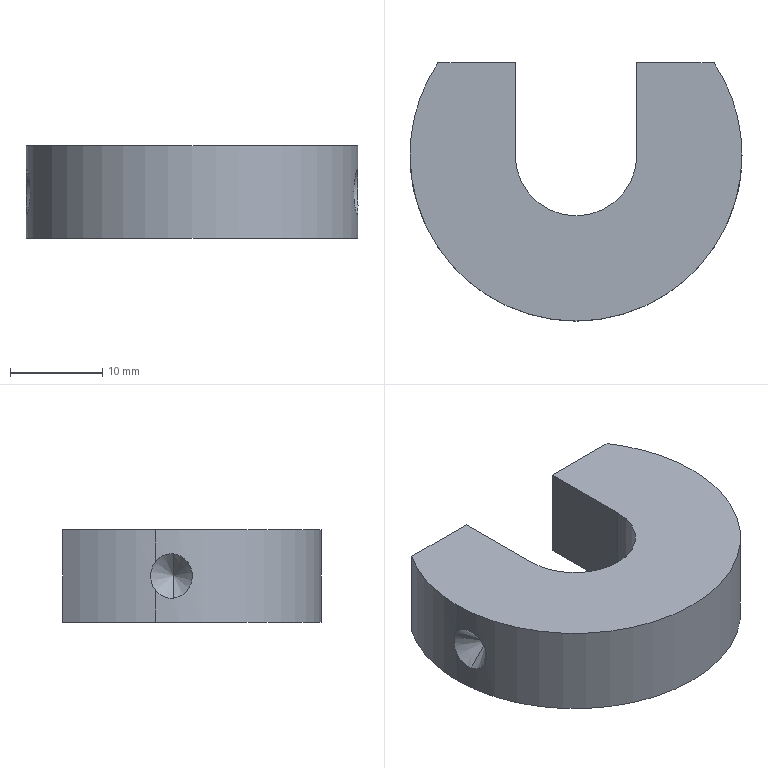Part | SolidWorks | features Extrusion 1, MirrorPattern 1, RevCut 1 | 1 solid | 14 faces | box 36 x 28 x 10 mm | volume 6463 mm3 | plane 6 | cone 4 | cylinder 4 | commonest cylinder face diameters 36 x3 13.2 x1